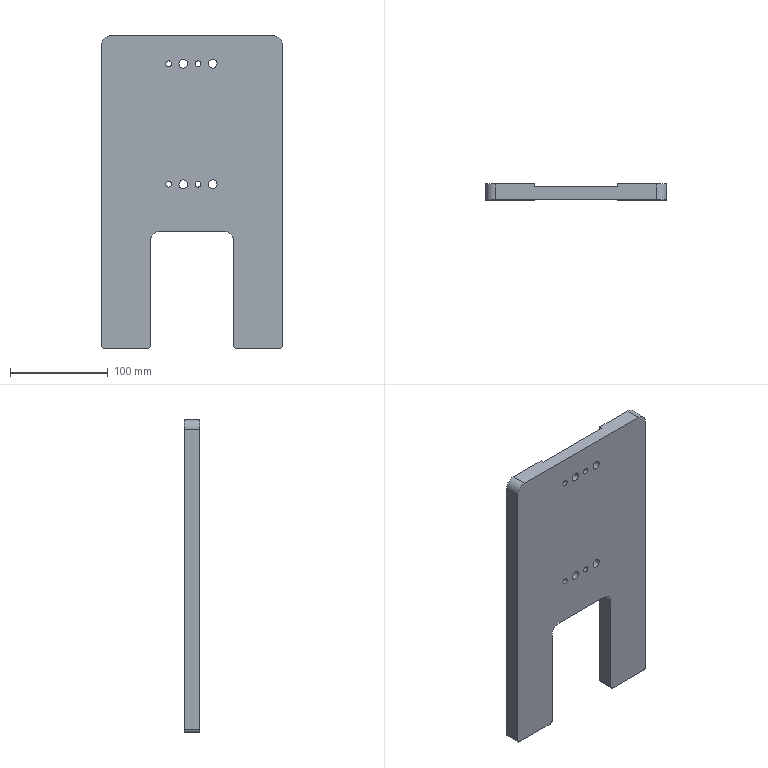Part | STEP file | SN10_006_005-01_PLACA | 1 solid | 28 faces | box 185 x 16 x 320 mm | volume 727969 mm3 | cylinder 16 | plane 12 | commonest cylinder face diameters 6 x8 9 x4 20 x4